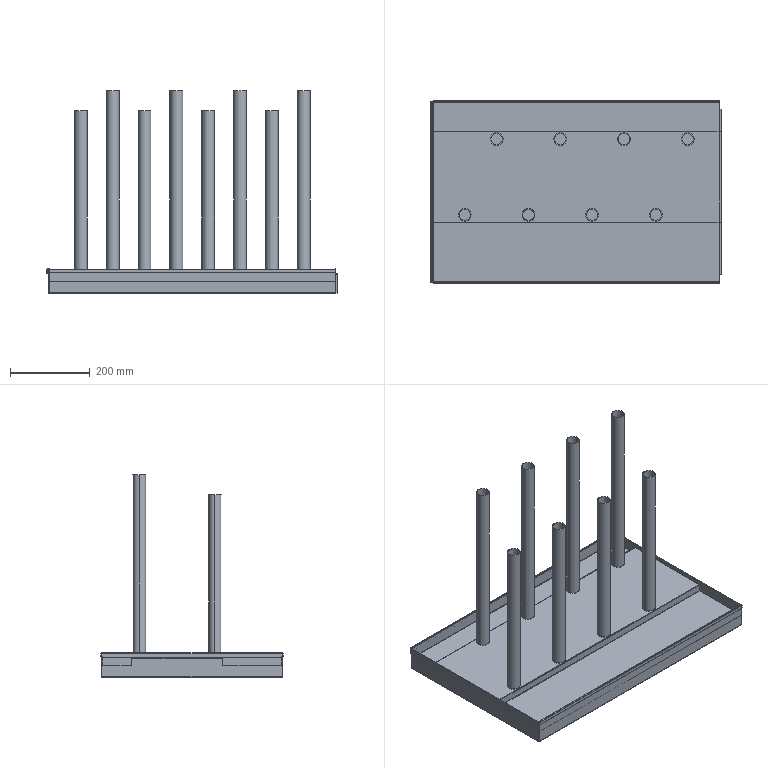Part | STEP file | RJWD-DY-0105--0001 | 10 solids | 226 faces | box 728.7 x 458 x 509.2 mm | volume 1538586 mm3 | plane 140 | cylinder 86 | commonest cylinder face diameters 32 x32 2.4 x18 29 x16 5 x8 8 x6 1.6 x2